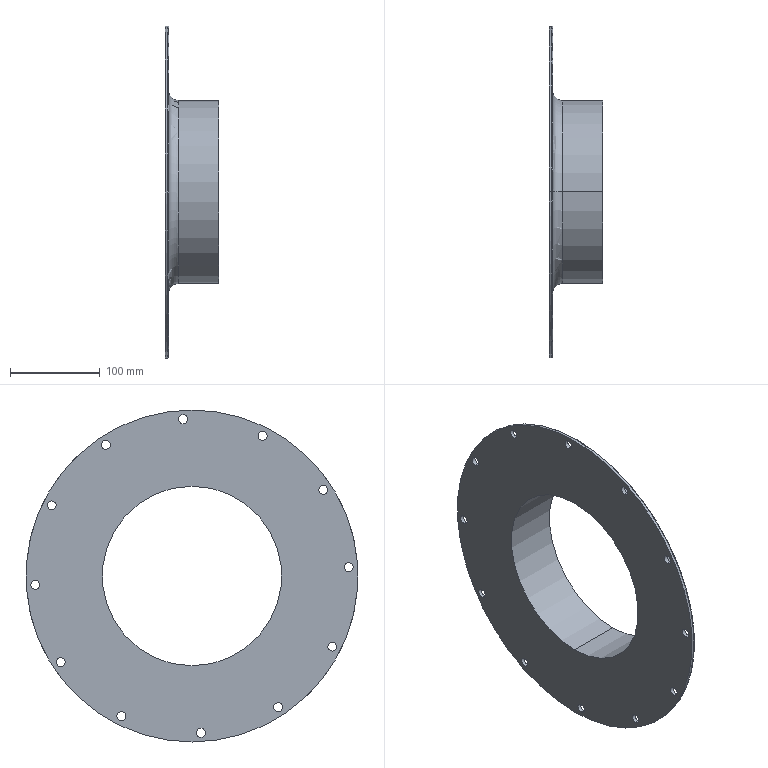Part | STEP file | wentylator blacha dodatkowaV11 | 1 solid | 61 faces | box 60 x 370 x 370 mm | volume 388519 mm3 | cylinder 30 | cone 24 | torus 4 | plane 3 | commonest cylinder face diameters 10 x24 200 x2 204 x2 370 x2